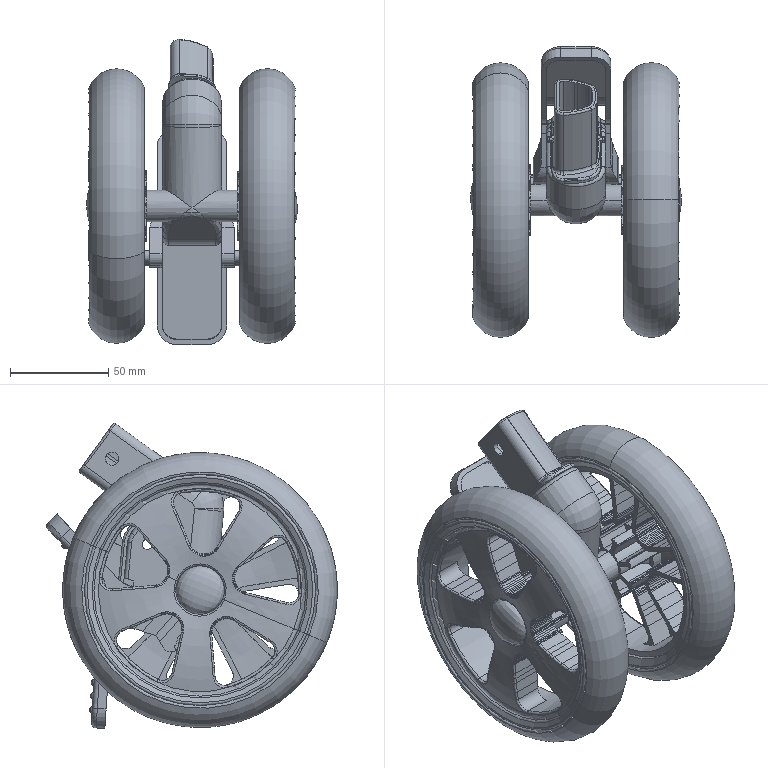Part | SolidWorks | 11 solids | 1970 faces | box 107.069 x 147.864 x 155.16 mm | volume 448012 mm3 | spline 932 | cylinder 535 | plane 288 | torus 143 | cone 56 | sphere 16 | commonest cylinder face diameters 1 x80 4 x50 2 x42 3 x33 10 x28 7 x26